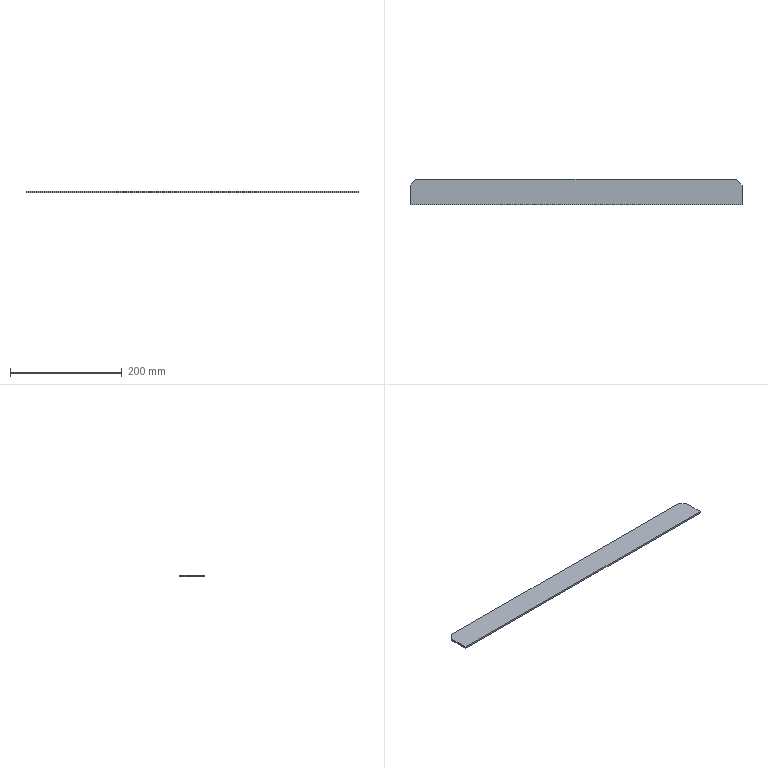Part | SolidWorks | features Chamfer 1, FlatPattern 1, SMBaseFlange 1, SheetMetal 1 | 1 solid | 8 faces | box 593.5 x 45 x 3.2 mm | volume 85144 mm3 | plane 8
STEP:
#1=CARTESIAN_POINT('',(593.5,35.,3.2));
#2=VERTEX_POINT('',#1);
#3=CARTESIAN_POINT('',(593.5,0.,3.2));
#4=VERTEX_POINT('',#3);
#5=CARTESIAN_POINT('',(593.5,45.,3.2));
#6=DIRECTION('',(0.,-1.,0.));
#7=VECTOR('',#6,1000.);
#8=LINE('',#5,#7);
#9=EDGE_CURVE('',#2,#4,#8,.T.);
#10=ORIENTED_EDGE('',*,*,#9,.F.);
#11=CARTESIAN_POINT('',(583.5,45.,3.2));
#12=VERTEX_POINT('',#11);
#13=CARTESIAN_POINT('',(593.5,35.,3.2));
#14=DIRECTION('',(-0.7071,0.7071,0.));
#15=VECTOR('',#14,1000.);
#16=LINE('',#13,#15);
#17=EDGE_CURVE('',#2,#12,#16,.T.);
#18=ORIENTED_EDGE('',*,*,#17,.T.);
#19=CARTESIAN_POINT('',(10.,45.,3.2));
#20=VERTEX_POINT('',#19);
#21=CARTESIAN_POINT('',(0.,45.,3.2));
#22=DIRECTION('',(1.,0.,0.));
#23=VECTOR('',#22,1000.);
#24=LINE('',#21,#23);
#25=EDGE_CURVE('',#20,#12,#24,.T.);
#26=ORIENTED_EDGE('',*,*,#25,.F.);
#27=CARTESIAN_POINT('',(0.,35.,3.2));
#28=VERTEX_POINT('',#27);
#29=CARTESIAN_POINT('',(0.,35.,3.2));
#30=DIRECTION('',(-0.7071,-0.7071,0.));
#31=VECTOR('',#30,1000.);
#32=LINE('',#29,#31);
#33=EDGE_CURVE('',#20,#28,#32,.T.);
#34=ORIENTED_EDGE('',*,*,#33,.T.);
#35=CARTESIAN_POINT('',(0.,0.,3.2));
#36=VERTEX_POINT('',#35);
#37=CARTESIAN_POINT('',(0.,45.,3.2));
#38=DIRECTION('',(0.,-1.,0.));
#39=VECTOR('',#38,1000.);
#40=LINE('',#37,#39);
#41=EDGE_CURVE('',#28,#36,#40,.T.);
#42=ORIENTED_EDGE('',*,*,#41,.T.);
#43=CARTESIAN_POINT('',(0.,0.,3.2));
#44=DIRECTION('',(1.,0.,0.));
#45=VECTOR('',#44,1000.);
#46=LINE('',#43,#45);
#47=EDGE_CURVE('',#36,#4,#46,.T.);
#48=ORIENTED_EDGE('',*,*,#47,.T.);
#49=EDGE_LOOP('',(#10,#18,#26,#34,#42,#48));
#50=FACE_OUTER_BOUND('',#49,.T.);
#51=CARTESIAN_POINT('',(0.,45.,3.2));
#52=DIRECTION('',(0.,0.,-1.));
#53=DIRECTION('',(-1.,0.,0.));
#54=AXIS2_PLACEMENT_3D('',#51,#52,#53);
#55=PLANE('',#54);
#56=ADVANCED_FACE('',(#50),#55,.F.);
#57=CARTESIAN_POINT('',(593.5,35.,0.));
#58=VERTEX_POINT('',#57);
#59=CARTESIAN_POINT('',(593.5,0.,0.));
#60=VERTEX_POINT('',#59);
#61=CARTESIAN_POINT('',(593.5,45.,0.));
#62=DIRECTION('',(0.,-1.,0.));
#63=VECTOR('',#62,1000.);
#64=LINE('',#61,#63);
#65=EDGE_CURVE('',#58,#60,#64,.T.);
#66=ORIENTED_EDGE('',*,*,#65,.F.);
#67=CARTESIAN_POINT('',(593.5,35.,3.2));
#68=DIRECTION('',(0.,0.,1.));
#69=VECTOR('',#68,1000.);
#70=LINE('',#67,#69);
#71=EDGE_CURVE('',#58,#2,#70,.T.);
#72=ORIENTED_EDGE('',*,*,#71,.T.);
#73=ORIENTED_EDGE('',*,*,#9,.T.);
#74=CARTESIAN_POINT('',(593.5,0.,0.));
#75=DIRECTION('',(0.,0.,1.));
#76=VECTOR('',#75,1000.);
#77=LINE('',#74,#76);
#78=EDGE_CURVE('',#60,#4,#77,.T.);
#79=ORIENTED_EDGE('',*,*,#78,.F.);
#80=EDGE_LOOP('',(#66,#72,#73,#79));
#81=FACE_OUTER_BOUND('',#80,.T.);
#82=CARTESIAN_POINT('',(593.5,45.,0.));
#83=DIRECTION('',(1.,0.,0.));
#84=DIRECTION('',(0.,0.,-1.));
#85=AXIS2_PLACEMENT_3D('',#82,#83,#84);
#86=PLANE('',#85);
#87=ADVANCED_FACE('',(#81),#86,.T.);
#88=CARTESIAN_POINT('',(10.,45.,0.));
#89=VERTEX_POINT('',#88);
#90=CARTESIAN_POINT('',(583.5,45.,0.));
#91=VERTEX_POINT('',#90);
#92=CARTESIAN_POINT('',(0.,45.,0.));
#93=DIRECTION('',(1.,0.,0.));
#94=VECTOR('',#93,1000.);
#95=LINE('',#92,#94);
#96=EDGE_CURVE('',#89,#91,#95,.T.);
#97=ORIENTED_EDGE('',*,*,#96,.T.);
#98=CARTESIAN_POINT('',(291.75,336.75,0.));
#99=DIRECTION('',(0.7071,-0.7071,0.));
#100=VECTOR('',#99,1000.);
#101=LINE('',#98,#100);
#102=EDGE_CURVE('',#91,#58,#101,.T.);
#103=ORIENTED_EDGE('',*,*,#102,.T.);
#104=ORIENTED_EDGE('',*,*,#65,.T.);
#105=CARTESIAN_POINT('',(0.,0.,0.));
#106=VERTEX_POINT('',#105);
#107=CARTESIAN_POINT('',(0.,0.,0.));
#108=DIRECTION('',(1.,0.,0.));
#109=VECTOR('',#108,1000.);
#110=LINE('',#107,#109);
#111=EDGE_CURVE('',#106,#60,#110,.T.);
#112=ORIENTED_EDGE('',*,*,#111,.F.);
#113=CARTESIAN_POINT('',(0.,35.,0.));
#114=VERTEX_POINT('',#113);
#115=CARTESIAN_POINT('',(0.,45.,0.));
#116=DIRECTION('',(0.,-1.,0.));
#117=VECTOR('',#116,1000.);
#118=LINE('',#115,#117);
#119=EDGE_CURVE('',#114,#106,#118,.T.);
#120=ORIENTED_EDGE('',*,*,#119,.F.);
#121=CARTESIAN_POINT('',(5.,40.,0.));
#122=DIRECTION('',(0.7071,0.7071,0.));
#123=VECTOR('',#122,1000.);
#124=LINE('',#121,#123);
#125=EDGE_CURVE('',#114,#89,#124,.T.);
#126=ORIENTED_EDGE('',*,*,#125,.T.);
#127=EDGE_LOOP('',(#97,#103,#104,#112,#120,#126));
#128=FACE_OUTER_BOUND('',#127,.T.);
#129=CARTESIAN_POINT('',(0.,45.,0.));
#130=DIRECTION('',(0.,0.,-1.));
#131=DIRECTION('',(-1.,0.,0.));
#132=AXIS2_PLACEMENT_3D('',#129,#130,#131);
#133=PLANE('',#132);
#134=ADVANCED_FACE('',(#128),#133,.T.);
#135=ORIENTED_EDGE('',*,*,#41,.F.);
#136=CARTESIAN_POINT('',(0.,35.,0.));
#137=DIRECTION('',(0.,0.,-1.));
#138=VECTOR('',#137,1000.);
#139=LINE('',#136,#138);
#140=EDGE_CURVE('',#28,#114,#139,.T.);
#141=ORIENTED_EDGE('',*,*,#140,.T.);
#142=ORIENTED_EDGE('',*,*,#119,.T.);
#143=CARTESIAN_POINT('',(0.,0.,3.2));
#144=DIRECTION('',(0.,0.,-1.));
#145=VECTOR('',#144,1000.);
#146=LINE('',#143,#145);
#147=EDGE_CURVE('',#36,#106,#146,.T.);
#148=ORIENTED_EDGE('',*,*,#147,.F.);
#149=EDGE_LOOP('',(#135,#141,#142,#148));
#150=FACE_OUTER_BOUND('',#149,.T.);
#151=CARTESIAN_POINT('',(0.,45.,3.2));
#152=DIRECTION('',(-1.,0.,0.));
#153=DIRECTION('',(0.,0.,1.));
#154=AXIS2_PLACEMENT_3D('',#151,#152,#153);
#155=PLANE('',#154);
#156=ADVANCED_FACE('',(#150),#155,.T.);
#157=ORIENTED_EDGE('',*,*,#25,.T.);
#158=CARTESIAN_POINT('',(583.5,45.,0.));
#159=DIRECTION('',(0.,0.,-1.));
#160=VECTOR('',#159,1000.);
#161=LINE('',#158,#160);
#162=EDGE_CURVE('',#12,#91,#161,.T.);
#163=ORIENTED_EDGE('',*,*,#162,.T.);
#164=ORIENTED_EDGE('',*,*,#96,.F.);
#165=CARTESIAN_POINT('',(10.,45.,3.2));
#166=DIRECTION('',(0.,0.,1.));
#167=VECTOR('',#166,1000.);
#168=LINE('',#165,#167);
#169=EDGE_CURVE('',#89,#20,#168,.T.);
#170=ORIENTED_EDGE('',*,*,#169,.T.);
#171=EDGE_LOOP('',(#157,#163,#164,#170));
#172=FACE_OUTER_BOUND('',#171,.T.);
#173=CARTESIAN_POINT('',(0.,45.,0.));
#174=DIRECTION('',(0.,-1.,0.));
#175=DIRECTION('',(-1.,0.,0.));
#176=AXIS2_PLACEMENT_3D('',#173,#174,#175);
#177=PLANE('',#176);
#178=ADVANCED_FACE('',(#172),#177,.F.);
#179=ORIENTED_EDGE('',*,*,#47,.F.);
#180=ORIENTED_EDGE('',*,*,#147,.T.);
#181=ORIENTED_EDGE('',*,*,#111,.T.);
#182=ORIENTED_EDGE('',*,*,#78,.T.);
#183=EDGE_LOOP('',(#179,#180,#181,#182));
#184=FACE_OUTER_BOUND('',#183,.T.);
#185=CARTESIAN_POINT('',(0.,0.,0.));
#186=DIRECTION('',(0.,-1.,0.));
#187=DIRECTION('',(-1.,0.,0.));
#188=AXIS2_PLACEMENT_3D('',#185,#186,#187);
#189=PLANE('',#188);
#190=ADVANCED_FACE('',(#184),#189,.T.);
#191=ORIENTED_EDGE('',*,*,#102,.F.);
#192=ORIENTED_EDGE('',*,*,#162,.F.);
#193=ORIENTED_EDGE('',*,*,#17,.F.);
#194=ORIENTED_EDGE('',*,*,#71,.F.);
#195=EDGE_LOOP('',(#191,#192,#193,#194));
#196=FACE_OUTER_BOUND('',#195,.T.);
#197=CARTESIAN_POINT('',(593.5,35.,0.));
#198=DIRECTION('',(0.7071,0.7071,0.));
#199=DIRECTION('',(0.,0.,-1.));
#200=AXIS2_PLACEMENT_3D('',#197,#198,#199);
#201=PLANE('',#200);
#202=ADVANCED_FACE('',(#196),#201,.T.);
#203=ORIENTED_EDGE('',*,*,#33,.F.);
#204=ORIENTED_EDGE('',*,*,#169,.F.);
#205=ORIENTED_EDGE('',*,*,#125,.F.);
#206=ORIENTED_EDGE('',*,*,#140,.F.);
#207=EDGE_LOOP('',(#203,#204,#205,#206));
#208=FACE_OUTER_BOUND('',#207,.T.);
#209=CARTESIAN_POINT('',(0.,35.,3.2));
#210=DIRECTION('',(-0.7071,0.7071,0.));
#211=DIRECTION('',(0.,0.,1.));
#212=AXIS2_PLACEMENT_3D('',#209,#210,#211);
#213=PLANE('',#212);
#214=ADVANCED_FACE('',(#208),#213,.T.);
#215=CLOSED_SHELL('',(#56,#87,#134,#156,#178,#190,#202,#214));
#216=MANIFOLD_SOLID_BREP('',#215);
#217=CARTESIAN_POINT('',(0.,0.,0.));
#218=DIRECTION('',(0.,0.,1.));
#219=DIRECTION('',(1.,0.,0.));
#220=AXIS2_PLACEMENT_3D('',#217,#218,#219);
#221=(LENGTH_UNIT()NAMED_UNIT(*)SI_UNIT(.MILLI.,.METRE.));
#222=UNCERTAINTY_MEASURE_WITH_UNIT(LENGTH_MEASURE(0.00001),#221,'','');
#223=(NAMED_UNIT(*)PLANE_ANGLE_UNIT()SI_UNIT($,.RADIAN.));
#224=(NAMED_UNIT(*)SI_UNIT($,.STERADIAN.)SOLID_ANGLE_UNIT());
#225=(GEOMETRIC_REPRESENTATION_CONTEXT(3)GLOBAL_UNCERTAINTY_ASSIGNED_CONTEXT((#222))GLOBAL_UNIT_ASSIGNED_CONTEXT((#221,#223,#224))REPRESENTATION_CONTEXT('',''));
#226=ADVANCED_BREP_SHAPE_REPRESENTATION('',(#216,#220),#225);